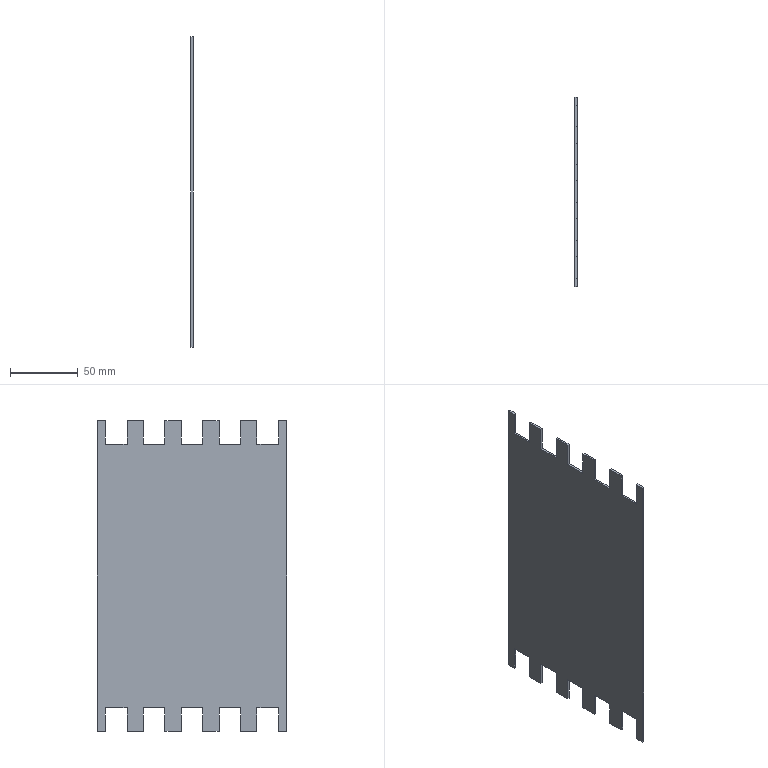Part | STEP file | A14-061 | 1 solid | 46 faces | box 1.5 x 140 x 230 mm | volume 44100 mm3 | plane 46